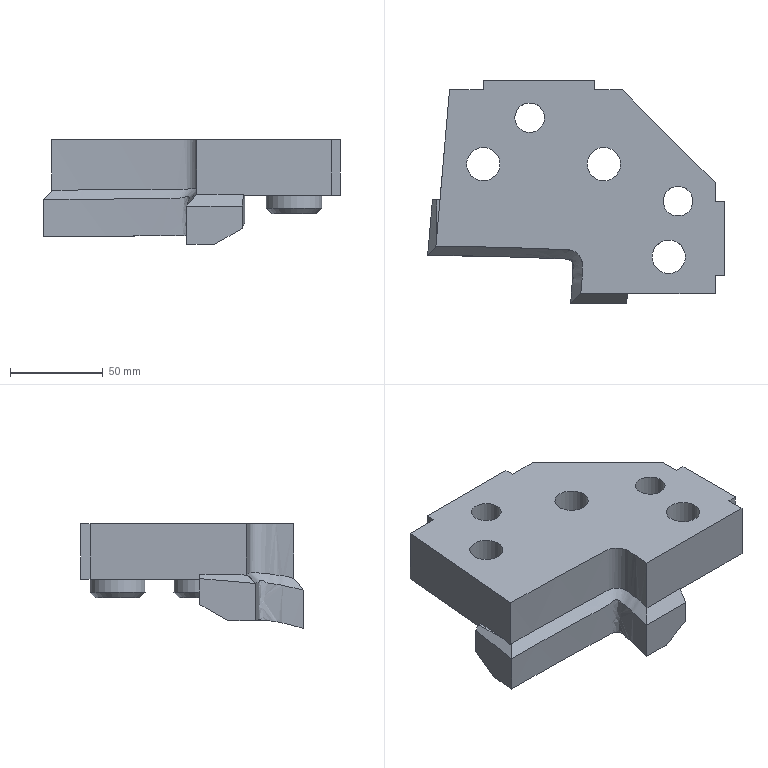Part | NX | features solid 2 | 1 solid | 43 faces | box 160.024 x 120 x 56.49 mm | volume 448318 mm3 | plane 25 | cylinder 10 | spline 6 | cone 2 | commonest cylinder face diameters 18 x3 26 x3 16 x2 30 x2